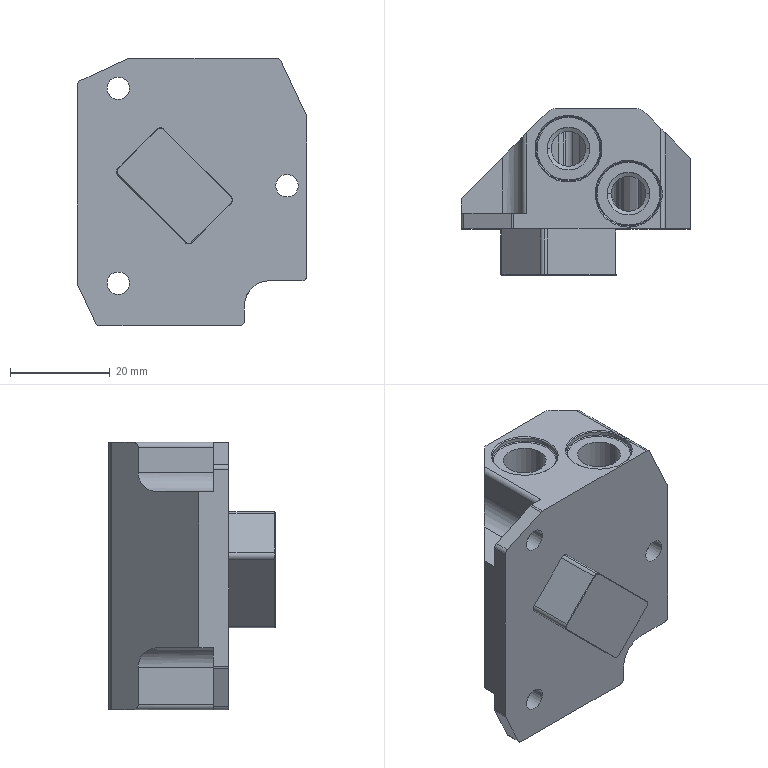Part | 1 solid | 154 faces | box 46 x 33.25 x 53.5 mm | volume 25757 mm3 | cylinder 66 | plane 54 | torus 13 | cone 12 | spline 6 | sphere 3 | commonest cylinder face diameters 2 x17 6 x10 13 x8 4 x7 4.5 x6 7 x4